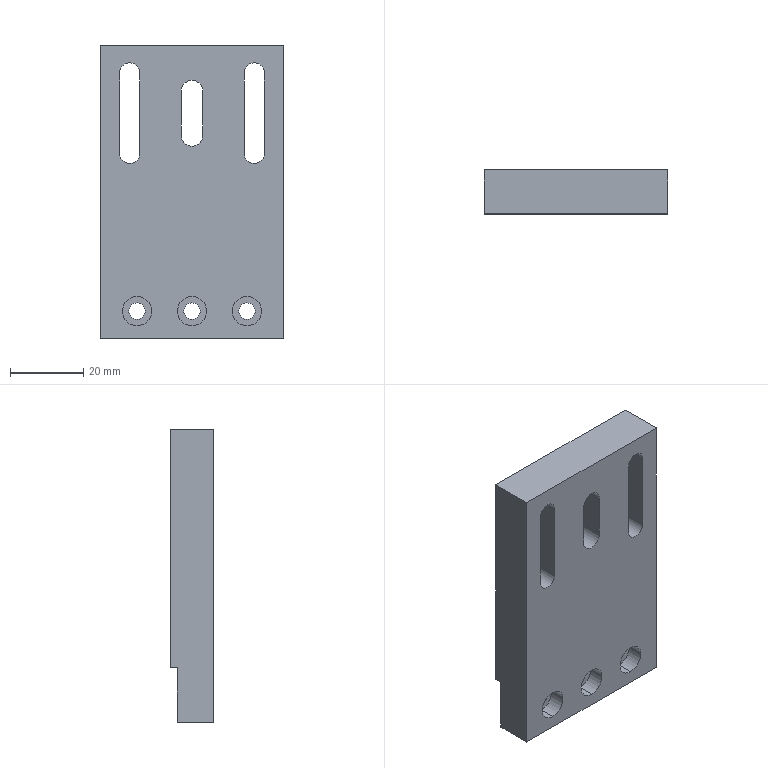Part | STEP file | 04-12 support plate | 1 solid | 50 faces | box 50 x 12 x 80 mm | volume 39354 mm3 | cylinder 27 | plane 23 | commonest cylinder face diameters 4.5 x6 5.5 x6 8 x6 10 x6 6 x3
STEP:
#1=CARTESIAN_POINT('',(17.,-6.,75.25));
#2=VERTEX_POINT('',#1);
#3=CARTESIAN_POINT('',(19.75,-6.,72.5));
#4=VERTEX_POINT('',#3);
#5=CARTESIAN_POINT('',(17.,-6.,72.5));
#6=DIRECTION('',(0.,1.,0.));
#7=DIRECTION('',(-1.,0.,0.));
#8=AXIS2_PLACEMENT_3D('',#5,#6,#7);
#9=CIRCLE('',#8,2.75);
#10=EDGE_CURVE('',#2,#4,#9,.T.);
#11=ORIENTED_EDGE('',*,*,#10,.F.);
#12=CARTESIAN_POINT('',(17.,1.,75.25));
#13=VERTEX_POINT('',#12);
#14=CARTESIAN_POINT('',(17.,-10.,75.25));
#15=DIRECTION('',(0.,1.,0.));
#16=VECTOR('',#15,1000.);
#17=LINE('',#14,#16);
#18=EDGE_CURVE('',#2,#13,#17,.T.);
#19=ORIENTED_EDGE('',*,*,#18,.T.);
#20=CARTESIAN_POINT('',(19.75,1.,72.5));
#21=VERTEX_POINT('',#20);
#22=CARTESIAN_POINT('',(17.,1.,72.5));
#23=DIRECTION('',(0.,-1.,0.));
#24=DIRECTION('',(0.,0.,-1.));
#25=AXIS2_PLACEMENT_3D('',#22,#23,#24);
#26=CIRCLE('',#25,2.75);
#27=EDGE_CURVE('',#21,#13,#26,.T.);
#28=ORIENTED_EDGE('',*,*,#27,.F.);
#29=CARTESIAN_POINT('',(19.75,-10.,72.5));
#30=DIRECTION('',(0.,1.,0.));
#31=VECTOR('',#30,1000.);
#32=LINE('',#29,#31);
#33=EDGE_CURVE('',#4,#21,#32,.T.);
#34=ORIENTED_EDGE('',*,*,#33,.F.);
#35=EDGE_LOOP('',(#11,#19,#28,#34));
#36=FACE_OUTER_BOUND('',#35,.T.);
#37=CARTESIAN_POINT('',(17.,-10.,72.5));
#38=DIRECTION('',(0.,1.,0.));
#39=DIRECTION('',(0.,0.,1.));
#40=AXIS2_PLACEMENT_3D('',#37,#38,#39);
#41=CYLINDRICAL_SURFACE('',#40,2.75);
#42=ADVANCED_FACE('',(#36),#41,.F.);
#43=CARTESIAN_POINT('',(-17.,-6.,75.25));
#44=VERTEX_POINT('',#43);
#45=CARTESIAN_POINT('',(-14.25,-6.,72.5));
#46=VERTEX_POINT('',#45);
#47=CARTESIAN_POINT('',(-17.,-6.,72.5));
#48=DIRECTION('',(0.,1.,0.));
#49=DIRECTION('',(-1.,0.,0.));
#50=AXIS2_PLACEMENT_3D('',#47,#48,#49);
#51=CIRCLE('',#50,2.75);
#52=EDGE_CURVE('',#44,#46,#51,.T.);
#53=ORIENTED_EDGE('',*,*,#52,.F.);
#54=CARTESIAN_POINT('',(-17.,1.,75.25));
#55=VERTEX_POINT('',#54);
#56=CARTESIAN_POINT('',(-17.,-10.,75.25));
#57=DIRECTION('',(0.,1.,0.));
#58=VECTOR('',#57,1000.);
#59=LINE('',#56,#58);
#60=EDGE_CURVE('',#44,#55,#59,.T.);
#61=ORIENTED_EDGE('',*,*,#60,.T.);
#62=CARTESIAN_POINT('',(-14.25,1.,72.5));
#63=VERTEX_POINT('',#62);
#64=CARTESIAN_POINT('',(-17.,1.,72.5));
#65=DIRECTION('',(0.,1.,0.));
#66=DIRECTION('',(0.,0.,1.));
#67=AXIS2_PLACEMENT_3D('',#64,#65,#66);
#68=CIRCLE('',#67,2.75);
#69=EDGE_CURVE('',#55,#63,#68,.T.);
#70=ORIENTED_EDGE('',*,*,#69,.T.);
#71=CARTESIAN_POINT('',(-14.25,-10.,72.5));
#72=DIRECTION('',(0.,1.,0.));
#73=VECTOR('',#72,1000.);
#74=LINE('',#71,#73);
#75=EDGE_CURVE('',#46,#63,#74,.T.);
#76=ORIENTED_EDGE('',*,*,#75,.F.);
#77=EDGE_LOOP('',(#53,#61,#70,#76));
#78=FACE_OUTER_BOUND('',#77,.T.);
#79=CARTESIAN_POINT('',(-17.,-10.,72.5));
#80=DIRECTION('',(0.,1.,0.));
#81=DIRECTION('',(0.,0.,1.));
#82=AXIS2_PLACEMENT_3D('',#79,#80,#81);
#83=CYLINDRICAL_SURFACE('',#82,2.75);
#84=ADVANCED_FACE('',(#78),#83,.F.);
#85=CARTESIAN_POINT('',(0.,-6.,70.5));
#86=VERTEX_POINT('',#85);
#87=CARTESIAN_POINT('',(3.,-6.,67.5));
#88=VERTEX_POINT('',#87);
#89=CARTESIAN_POINT('',(0.,-6.,67.5));
#90=DIRECTION('',(0.,1.,0.));
#91=DIRECTION('',(-1.,0.,0.));
#92=AXIS2_PLACEMENT_3D('',#89,#90,#91);
#93=CIRCLE('',#92,3.);
#94=EDGE_CURVE('',#86,#88,#93,.T.);
#95=ORIENTED_EDGE('',*,*,#94,.F.);
#96=CARTESIAN_POINT('',(0.,6.,70.5));
#97=VERTEX_POINT('',#96);
#98=CARTESIAN_POINT('',(0.,-10.,70.5));
#99=DIRECTION('',(0.,1.,0.));
#100=VECTOR('',#99,1000.);
#101=LINE('',#98,#100);
#102=EDGE_CURVE('',#86,#97,#101,.T.);
#103=ORIENTED_EDGE('',*,*,#102,.T.);
#104=CARTESIAN_POINT('',(3.,6.,67.5));
#105=VERTEX_POINT('',#104);
#106=CARTESIAN_POINT('',(0.,6.,67.5));
#107=DIRECTION('',(0.,-1.,0.));
#108=DIRECTION('',(0.,0.,-1.));
#109=AXIS2_PLACEMENT_3D('',#106,#107,#108);
#110=CIRCLE('',#109,3.);
#111=EDGE_CURVE('',#105,#97,#110,.T.);
#112=ORIENTED_EDGE('',*,*,#111,.F.);
#113=CARTESIAN_POINT('',(3.,-10.,67.5));
#114=DIRECTION('',(0.,1.,0.));
#115=VECTOR('',#114,1000.);
#116=LINE('',#113,#115);
#117=EDGE_CURVE('',#88,#105,#116,.T.);
#118=ORIENTED_EDGE('',*,*,#117,.F.);
#119=EDGE_LOOP('',(#95,#103,#112,#118));
#120=FACE_OUTER_BOUND('',#119,.T.);
#121=CARTESIAN_POINT('',(0.,-10.,67.5));
#122=DIRECTION('',(0.,1.,0.));
#123=DIRECTION('',(0.,0.,1.));
#124=AXIS2_PLACEMENT_3D('',#121,#122,#123);
#125=CYLINDRICAL_SURFACE('',#124,3.);
#126=ADVANCED_FACE('',(#120),#125,.F.);
#127=CARTESIAN_POINT('',(17.,1.,77.5));
#128=VERTEX_POINT('',#127);
#129=CARTESIAN_POINT('',(22.,1.,72.5));
#130=VERTEX_POINT('',#129);
#131=CARTESIAN_POINT('',(17.,1.,72.5));
#132=DIRECTION('',(0.,1.,0.));
#133=DIRECTION('',(0.,0.,-1.));
#134=AXIS2_PLACEMENT_3D('',#131,#132,#133);
#135=CIRCLE('',#134,5.);
#136=EDGE_CURVE('',#128,#130,#135,.T.);
#137=ORIENTED_EDGE('',*,*,#136,.F.);
#138=CARTESIAN_POINT('',(17.,6.,77.5));
#139=VERTEX_POINT('',#138);
#140=CARTESIAN_POINT('',(17.,1.,77.5));
#141=DIRECTION('',(0.,1.,0.));
#142=VECTOR('',#141,1000.);
#143=LINE('',#140,#142);
#144=EDGE_CURVE('',#128,#139,#143,.T.);
#145=ORIENTED_EDGE('',*,*,#144,.T.);
#146=CARTESIAN_POINT('',(22.,6.,72.5));
#147=VERTEX_POINT('',#146);
#148=CARTESIAN_POINT('',(17.,6.,72.5));
#149=DIRECTION('',(0.,1.,0.));
#150=DIRECTION('',(0.,0.,-1.));
#151=AXIS2_PLACEMENT_3D('',#148,#149,#150);
#152=CIRCLE('',#151,5.);
#153=EDGE_CURVE('',#139,#147,#152,.T.);
#154=ORIENTED_EDGE('',*,*,#153,.T.);
#155=CARTESIAN_POINT('',(22.,1.,72.5));
#156=DIRECTION('',(0.,1.,0.));
#157=VECTOR('',#156,1000.);
#158=LINE('',#155,#157);
#159=EDGE_CURVE('',#130,#147,#158,.T.);
#160=ORIENTED_EDGE('',*,*,#159,.F.);
#161=EDGE_LOOP('',(#137,#145,#154,#160));
#162=FACE_OUTER_BOUND('',#161,.T.);
#163=CARTESIAN_POINT('',(17.,1.,72.5));
#164=DIRECTION('',(0.,1.,0.));
#165=DIRECTION('',(0.,0.,1.));
#166=AXIS2_PLACEMENT_3D('',#163,#164,#165);
#167=CYLINDRICAL_SURFACE('',#166,5.);
#168=ADVANCED_FACE('',(#162),#167,.F.);
#169=CARTESIAN_POINT('',(-17.,1.,77.5));
#170=VERTEX_POINT('',#169);
#171=CARTESIAN_POINT('',(-12.,1.,72.5));
#172=VERTEX_POINT('',#171);
#173=CARTESIAN_POINT('',(-17.,1.,72.5));
#174=DIRECTION('',(0.,1.,0.));
#175=DIRECTION('',(0.,0.,1.));
#176=AXIS2_PLACEMENT_3D('',#173,#174,#175);
#177=CIRCLE('',#176,5.);
#178=EDGE_CURVE('',#170,#172,#177,.T.);
#179=ORIENTED_EDGE('',*,*,#178,.F.);
#180=CARTESIAN_POINT('',(-17.,6.,77.5));
#181=VERTEX_POINT('',#180);
#182=CARTESIAN_POINT('',(-17.,1.,77.5));
#183=DIRECTION('',(0.,1.,0.));
#184=VECTOR('',#183,1000.);
#185=LINE('',#182,#184);
#186=EDGE_CURVE('',#170,#181,#185,.T.);
#187=ORIENTED_EDGE('',*,*,#186,.T.);
#188=CARTESIAN_POINT('',(-12.,6.,72.5));
#189=VERTEX_POINT('',#188);
#190=CARTESIAN_POINT('',(-17.,6.,72.5));
#191=DIRECTION('',(0.,1.,0.));
#192=DIRECTION('',(0.,0.,1.));
#193=AXIS2_PLACEMENT_3D('',#190,#191,#192);
#194=CIRCLE('',#193,5.);
#195=EDGE_CURVE('',#181,#189,#194,.T.);
#196=ORIENTED_EDGE('',*,*,#195,.T.);
#197=CARTESIAN_POINT('',(-12.,1.,72.5));
#198=DIRECTION('',(0.,1.,0.));
#199=VECTOR('',#198,1000.);
#200=LINE('',#197,#199);
#201=EDGE_CURVE('',#172,#189,#200,.T.);
#202=ORIENTED_EDGE('',*,*,#201,.F.);
#203=EDGE_LOOP('',(#179,#187,#196,#202));
#204=FACE_OUTER_BOUND('',#203,.T.);
#205=CARTESIAN_POINT('',(-17.,1.,72.5));
#206=DIRECTION('',(0.,1.,0.));
#207=DIRECTION('',(0.,0.,1.));
#208=AXIS2_PLACEMENT_3D('',#205,#206,#207);
#209=CYLINDRICAL_SURFACE('',#208,5.);
#210=ADVANCED_FACE('',(#204),#209,.F.);
#211=CARTESIAN_POINT('',(15.,-1.6,11.5));
#212=VERTEX_POINT('',#211);
#213=CARTESIAN_POINT('',(15.,-1.6,3.5));
#214=VERTEX_POINT('',#213);
#215=CARTESIAN_POINT('',(15.,-1.6,7.5));
#216=DIRECTION('',(0.,-1.,0.));
#217=DIRECTION('',(0.,0.,-1.));
#218=AXIS2_PLACEMENT_3D('',#215,#216,#217);
#219=CIRCLE('',#218,4.);
#220=EDGE_CURVE('',#212,#214,#219,.T.);
#221=ORIENTED_EDGE('',*,*,#220,.F.);
#222=CARTESIAN_POINT('',(15.,-6.,11.5));
#223=VERTEX_POINT('',#222);
#224=CARTESIAN_POINT('',(15.,-6.,11.5));
#225=DIRECTION('',(0.,-1.,0.));
#226=VECTOR('',#225,1000.);
#227=LINE('',#224,#226);
#228=EDGE_CURVE('',#212,#223,#227,.T.);
#229=ORIENTED_EDGE('',*,*,#228,.T.);
#230=CARTESIAN_POINT('',(15.,-6.,3.5));
#231=VERTEX_POINT('',#230);
#232=CARTESIAN_POINT('',(15.,-6.,7.5));
#233=DIRECTION('',(0.,-1.,0.));
#234=DIRECTION('',(0.,0.,-1.));
#235=AXIS2_PLACEMENT_3D('',#232,#233,#234);
#236=CIRCLE('',#235,4.);
#237=EDGE_CURVE('',#223,#231,#236,.T.);
#238=ORIENTED_EDGE('',*,*,#237,.T.);
#239=CARTESIAN_POINT('',(15.,-6.,3.5));
#240=DIRECTION('',(0.,-1.,0.));
#241=VECTOR('',#240,1000.);
#242=LINE('',#239,#241);
#243=EDGE_CURVE('',#214,#231,#242,.T.);
#244=ORIENTED_EDGE('',*,*,#243,.F.);
#245=EDGE_LOOP('',(#221,#229,#238,#244));
#246=FACE_OUTER_BOUND('',#245,.T.);
#247=CARTESIAN_POINT('',(15.,-6.,7.5));
#248=DIRECTION('',(0.,-1.,0.));
#249=DIRECTION('',(0.,0.,-1.));
#250=AXIS2_PLACEMENT_3D('',#247,#248,#249);
#251=CYLINDRICAL_SURFACE('',#250,4.);
#252=ADVANCED_FACE('',(#246),#251,.F.);
#253=CARTESIAN_POINT('',(15.,4.,9.75));
#254=VERTEX_POINT('',#253);
#255=CARTESIAN_POINT('',(15.,4.,5.25));
#256=VERTEX_POINT('',#255);
#257=CARTESIAN_POINT('',(15.,4.,7.5));
#258=DIRECTION('',(0.,-1.,0.));
#259=DIRECTION('',(1.,0.,0.));
#260=AXIS2_PLACEMENT_3D('',#257,#258,#259);
#261=CIRCLE('',#260,2.25);
#262=EDGE_CURVE('',#254,#256,#261,.T.);
#263=ORIENTED_EDGE('',*,*,#262,.F.);
#264=CARTESIAN_POINT('',(15.,-1.6,9.75));
#265=VERTEX_POINT('',#264);
#266=CARTESIAN_POINT('',(15.,-6.,9.75));
#267=DIRECTION('',(0.,-1.,0.));
#268=VECTOR('',#267,1000.);
#269=LINE('',#266,#268);
#270=EDGE_CURVE('',#254,#265,#269,.T.);
#271=ORIENTED_EDGE('',*,*,#270,.T.);
#272=CARTESIAN_POINT('',(15.,-1.6,5.25));
#273=VERTEX_POINT('',#272);
#274=CARTESIAN_POINT('',(15.,-1.6,7.5));
#275=DIRECTION('',(0.,-1.,0.));
#276=DIRECTION('',(0.,0.,-1.));
#277=AXIS2_PLACEMENT_3D('',#274,#275,#276);
#278=CIRCLE('',#277,2.25);
#279=EDGE_CURVE('',#265,#273,#278,.T.);
#280=ORIENTED_EDGE('',*,*,#279,.T.);
#281=CARTESIAN_POINT('',(15.,-6.,5.25));
#282=DIRECTION('',(0.,-1.,0.));
#283=VECTOR('',#282,1000.);
#284=LINE('',#281,#283);
#285=EDGE_CURVE('',#256,#273,#284,.T.);
#286=ORIENTED_EDGE('',*,*,#285,.F.);
#287=EDGE_LOOP('',(#263,#271,#280,#286));
#288=FACE_OUTER_BOUND('',#287,.T.);
#289=CARTESIAN_POINT('',(15.,-6.,7.5));
#290=DIRECTION('',(0.,-1.,0.));
#291=DIRECTION('',(0.,0.,-1.));
#292=AXIS2_PLACEMENT_3D('',#289,#290,#291);
#293=CYLINDRICAL_SURFACE('',#292,2.25);
#294=ADVANCED_FACE('',(#288),#293,.F.);
#295=CARTESIAN_POINT('',(0.,-1.6,11.5));
#296=VERTEX_POINT('',#295);
#297=CARTESIAN_POINT('',(0.,-1.6,3.5));
#298=VERTEX_POINT('',#297);
#299=CARTESIAN_POINT('',(0.,-1.6,7.5));
#300=DIRECTION('',(0.,-1.,0.));
#301=DIRECTION('',(0.,0.,-1.));
#302=AXIS2_PLACEMENT_3D('',#299,#300,#301);
#303=CIRCLE('',#302,4.);
#304=EDGE_CURVE('',#296,#298,#303,.T.);
#305=ORIENTED_EDGE('',*,*,#304,.F.);
#306=CARTESIAN_POINT('',(0.,-6.,11.5));
#307=VERTEX_POINT('',#306);
#308=CARTESIAN_POINT('',(0.,-6.,11.5));
#309=DIRECTION('',(0.,-1.,0.));
#310=VECTOR('',#309,1000.);
#311=LINE('',#308,#310);
#312=EDGE_CURVE('',#296,#307,#311,.T.);
#313=ORIENTED_EDGE('',*,*,#312,.T.);
#314=CARTESIAN_POINT('',(0.,-6.,3.5));
#315=VERTEX_POINT('',#314);
#316=CARTESIAN_POINT('',(0.,-6.,7.5));
#317=DIRECTION('',(0.,-1.,0.));
#318=DIRECTION('',(0.,0.,-1.));
#319=AXIS2_PLACEMENT_3D('',#316,#317,#318);
#320=CIRCLE('',#319,4.);
#321=EDGE_CURVE('',#307,#315,#320,.T.);
#322=ORIENTED_EDGE('',*,*,#321,.T.);
#323=CARTESIAN_POINT('',(0.,-6.,3.5));
#324=DIRECTION('',(0.,-1.,0.));
#325=VECTOR('',#324,1000.);
#326=LINE('',#323,#325);
#327=EDGE_CURVE('',#298,#315,#326,.T.);
#328=ORIENTED_EDGE('',*,*,#327,.F.);
#329=EDGE_LOOP('',(#305,#313,#322,#328));
#330=FACE_OUTER_BOUND('',#329,.T.);
#331=CARTESIAN_POINT('',(0.,-6.,7.5));
#332=DIRECTION('',(0.,-1.,0.));
#333=DIRECTION('',(0.,0.,-1.));
#334=AXIS2_PLACEMENT_3D('',#331,#332,#333);
#335=CYLINDRICAL_SURFACE('',#334,4.);
#336=ADVANCED_FACE('',(#330),#335,.F.);
#337=CARTESIAN_POINT('',(0.,4.,9.75));
#338=VERTEX_POINT('',#337);
#339=CARTESIAN_POINT('',(0.,4.,5.25));
#340=VERTEX_POINT('',#339);
#341=CARTESIAN_POINT('',(0.,4.,7.5));
#342=DIRECTION('',(0.,-1.,0.));
#343=DIRECTION('',(1.,0.,0.));
#344=AXIS2_PLACEMENT_3D('',#341,#342,#343);
#345=CIRCLE('',#344,2.25);
#346=EDGE_CURVE('',#338,#340,#345,.T.);
#347=ORIENTED_EDGE('',*,*,#346,.F.);
#348=CARTESIAN_POINT('',(0.,-1.6,9.75));
#349=VERTEX_POINT('',#348);
#350=CARTESIAN_POINT('',(0.,-6.,9.75));
#351=DIRECTION('',(0.,-1.,0.));
#352=VECTOR('',#351,1000.);
#353=LINE('',#350,#352);
#354=EDGE_CURVE('',#338,#349,#353,.T.);
#355=ORIENTED_EDGE('',*,*,#354,.T.);
#356=CARTESIAN_POINT('',(0.,-1.6,5.25));
#357=VERTEX_POINT('',#356);
#358=CARTESIAN_POINT('',(0.,-1.6,7.5));
#359=DIRECTION('',(0.,-1.,0.));
#360=DIRECTION('',(0.,0.,-1.));
#361=AXIS2_PLACEMENT_3D('',#358,#359,#360);
#362=CIRCLE('',#361,2.25);
#363=EDGE_CURVE('',#349,#357,#362,.T.);
#364=ORIENTED_EDGE('',*,*,#363,.T.);
#365=CARTESIAN_POINT('',(0.,-6.,5.25));
#366=DIRECTION('',(0.,-1.,0.));
#367=VECTOR('',#366,1000.);
#368=LINE('',#365,#367);
#369=EDGE_CURVE('',#340,#357,#368,.T.);
#370=ORIENTED_EDGE('',*,*,#369,.F.);
#371=EDGE_LOOP('',(#347,#355,#364,#370));
#372=FACE_OUTER_BOUND('',#371,.T.);
#373=CARTESIAN_POINT('',(0.,-6.,7.5));
#374=DIRECTION('',(0.,-1.,0.));
#375=DIRECTION('',(0.,0.,-1.));
#376=AXIS2_PLACEMENT_3D('',#373,#374,#375);
#377=CYLINDRICAL_SURFACE('',#376,2.25);
#378=ADVANCED_FACE('',(#372),#377,.F.);
#379=CARTESIAN_POINT('',(-15.,-1.6,11.5));
#380=VERTEX_POINT('',#379);
#381=CARTESIAN_POINT('',(-15.,-1.6,3.5));
#382=VERTEX_POINT('',#381);
#383=CARTESIAN_POINT('',(-15.,-1.6,7.5));
#384=DIRECTION('',(0.,-1.,0.));
#385=DIRECTION('',(0.,0.,-1.));
#386=AXIS2_PLACEMENT_3D('',#383,#384,#385);
#387=CIRCLE('',#386,4.);
#388=EDGE_CURVE('',#380,#382,#387,.T.);
#389=ORIENTED_EDGE('',*,*,#388,.F.);
#390=CARTESIAN_POINT('',(-15.,-6.,11.5));
#391=VERTEX_POINT('',#390);
#392=CARTESIAN_POINT('',(-15.,-6.,11.5));
#393=DIRECTION('',(0.,-1.,0.));
#394=VECTOR('',#393,1000.);
#395=LINE('',#392,#394);
#396=EDGE_CURVE('',#380,#391,#395,.T.);
#397=ORIENTED_EDGE('',*,*,#396,.T.);
#398=CARTESIAN_POINT('',(-15.,-6.,3.5));
#399=VERTEX_POINT('',#398);
#400=CARTESIAN_POINT('',(-15.,-6.,7.5));
#401=DIRECTION('',(0.,-1.,0.));
#402=DIRECTION('',(0.,0.,-1.));
#403=AXIS2_PLACEMENT_3D('',#400,#401,#402);
#404=CIRCLE('',#403,4.);
#405=EDGE_CURVE('',#391,#399,#404,.T.);
#406=ORIENTED_EDGE('',*,*,#405,.T.);
#407=CARTESIAN_POINT('',(-15.,-6.,3.5));
#408=DIRECTION('',(0.,-1.,0.));
#409=VECTOR('',#408,1000.);
#410=LINE('',#407,#409);
#411=EDGE_CURVE('',#382,#399,#410,.T.);
#412=ORIENTED_EDGE('',*,*,#411,.F.);
#413=EDGE_LOOP('',(#389,#397,#406,#412));
#414=FACE_OUTER_BOUND('',#413,.T.);
#415=CARTESIAN_POINT('',(-15.,-6.,7.5));
#416=DIRECTION('',(0.,-1.,0.));
#417=DIRECTION('',(0.,0.,-1.));
#418=AXIS2_PLACEMENT_3D('',#415,#416,#417);
#419=CYLINDRICAL_SURFACE('',#418,4.);
#420=ADVANCED_FACE('',(#414),#419,.F.);
#421=CARTESIAN_POINT('',(-15.,4.,9.75));
#422=VERTEX_POINT('',#421);
#423=CARTESIAN_POINT('',(-15.,4.,5.25));
#424=VERTEX_POINT('',#423);
#425=CARTESIAN_POINT('',(-15.,4.,7.5));
#426=DIRECTION('',(0.,-1.,0.));
#427=DIRECTION('',(1.,0.,0.));
#428=AXIS2_PLACEMENT_3D('',#425,#426,#427);
#429=CIRCLE('',#428,2.25);
#430=EDGE_CURVE('',#422,#424,#429,.T.);
#431=ORIENTED_EDGE('',*,*,#430,.F.);
#432=CARTESIAN_POINT('',(-15.,-1.6,9.75));
#433=VERTEX_POINT('',#432);
#434=CARTESIAN_POINT('',(-15.,-6.,9.75));
#435=DIRECTION('',(0.,-1.,0.));
#436=VECTOR('',#435,1000.);
#437=LINE('',#434,#436);
#438=EDGE_CURVE('',#422,#433,#437,.T.);
#439=ORIENTED_EDGE('',*,*,#438,.T.);
#440=CARTESIAN_POINT('',(-15.,-1.6,5.25));
#441=VERTEX_POINT('',#440);
#442=CARTESIAN_POINT('',(-15.,-1.6,7.5));
#443=DIRECTION('',(0.,-1.,0.));
#444=DIRECTION('',(0.,0.,-1.));
#445=AXIS2_PLACEMENT_3D('',#442,#443,#444);
#446=CIRCLE('',#445,2.25);
#447=EDGE_CURVE('',#433,#441,#446,.T.);
#448=ORIENTED_EDGE('',*,*,#447,.T.);
#449=CARTESIAN_POINT('',(-15.,-6.,5.25));
#450=DIRECTION('',(0.,-1.,0.));
#451=VECTOR('',#450,1000.);
#452=LINE('',#449,#451);
#453=EDGE_CURVE('',#424,#441,#452,.T.);
#454=ORIENTED_EDGE('',*,*,#453,.F.);
#455=EDGE_LOOP('',(#431,#439,#448,#454));
#456=FACE_OUTER_BOUND('',#455,.T.);
#457=CARTESIAN_POINT('',(-15.,-6.,7.5));
#458=DIRECTION('',(0.,-1.,0.));
#459=DIRECTION('',(0.,0.,-1.));
#460=AXIS2_PLACEMENT_3D('',#457,#458,#459);
#461=CYLINDRICAL_SURFACE('',#460,2.25);
#462=ADVANCED_FACE('',(#456),#461,.F.);
#463=CARTESIAN_POINT('',(25.,-6.,0.));
#464=VERTEX_POINT('',#463);
#465=CARTESIAN_POINT('',(25.,4.,0.));
#466=VERTEX_POINT('',#465);
#467=CARTESIAN_POINT('',(25.,6.,0.));
#468=DIRECTION('',(0.,1.,0.));
#469=VECTOR('',#468,1000.);
#470=LINE('',#467,#469);
#471=EDGE_CURVE('',#464,#466,#470,.T.);
#472=ORIENTED_EDGE('',*,*,#471,.T.);
#473=CARTESIAN_POINT('',(25.,4.,15.));
#474=VERTEX_POINT('',#473);
#475=CARTESIAN_POINT('',(25.,4.,0.));
#476=DIRECTION('',(0.,0.,-1.));
#477=VECTOR('',#476,1000.);
#478=LINE('',#475,#477);
#479=EDGE_CURVE('',#474,#466,#478,.T.);
#480=ORIENTED_EDGE('',*,*,#479,.F.);
#481=CARTESIAN_POINT('',(25.,6.,15.));
#482=VERTEX_POINT('',#481);
#483=CARTESIAN_POINT('',(25.,6.,15.));
#484=DIRECTION('',(0.,-1.,0.));
#485=VECTOR('',#484,1000.);
#486=LINE('',#483,#485);
#487=EDGE_CURVE('',#482,#474,#486,.T.);
#488=ORIENTED_EDGE('',*,*,#487,.F.);
#489=CARTESIAN_POINT('',(25.,6.,80.));
#490=VERTEX_POINT('',#489);
#491=CARTESIAN_POINT('',(25.,6.,80.));
#492=DIRECTION('',(0.,0.,-1.));
#493=VECTOR('',#492,1000.);
#494=LINE('',#491,#493);
#495=EDGE_CURVE('',#490,#482,#494,.T.);
#496=ORIENTED_EDGE('',*,*,#495,.F.);
#497=CARTESIAN_POINT('',(25.,-6.,80.));
#498=VERTEX_POINT('',#497);
#499=CARTESIAN_POINT('',(25.,6.,80.));
#500=DIRECTION('',(0.,1.,0.));
#501=VECTOR('',#500,1000.);
#502=LINE('',#499,#501);
#503=EDGE_CURVE('',#498,#490,#502,.T.);
#504=ORIENTED_EDGE('',*,*,#503,.F.);
#505=CARTESIAN_POINT('',(25.,-6.,80.));
#506=DIRECTION('',(0.,0.,-1.));
#507=VECTOR('',#506,1000.);
#508=LINE('',#505,#507);
#509=EDGE_CURVE('',#498,#464,#508,.T.);
#510=ORIENTED_EDGE('',*,*,#509,.T.);
#511=EDGE_LOOP('',(#472,#480,#488,#496,#504,#510));
#512=FACE_OUTER_BOUND('',#511,.T.);
#513=CARTESIAN_POINT('',(25.,6.,80.));
#514=DIRECTION('',(-1.,0.,0.));
#515=DIRECTION('',(0.,-1.,0.));
#516=AXIS2_PLACEMENT_3D('',#513,#514,#515);
#517=PLANE('',#516);
#518=ADVANCED_FACE('',(#512),#517,.F.);
#519=CARTESIAN_POINT('',(-3.,6.,67.5));
#520=VERTEX_POINT('',#519);
#521=CARTESIAN_POINT('',(-3.,6.,55.5));
#522=VERTEX_POINT('',#521);
#523=CARTESIAN_POINT('',(-3.,6.,80.));
#524=DIRECTION('',(0.,0.,-1.));
#525=VECTOR('',#524,1000.);
#526=LINE('',#523,#525);
#527=EDGE_CURVE('',#520,#522,#526,.T.);
#528=ORIENTED_EDGE('',*,*,#527,.T.);
#529=CARTESIAN_POINT('',(3.,6.,55.5));
#530=VERTEX_POINT('',#529);
#531=CARTESIAN_POINT('',(0.,6.,55.5));
#532=DIRECTION('',(0.,-1.,0.));
#533=DIRECTION('',(0.,0.,-1.));
#534=AXIS2_PLACEMENT_3D('',#531,#532,#533);
#535=CIRCLE('',#534,3.);
#536=EDGE_CURVE('',#522,#530,#535,.T.);
#537=ORIENTED_EDGE('',*,*,#536,.T.);
#538=CARTESIAN_POINT('',(3.,6.,80.));
#539=DIRECTION('',(0.,0.,1.));
#540=VECTOR('',#539,1000.);
#541=LINE('',#538,#540);
#542=EDGE_CURVE('',#530,#105,#541,.T.);
#543=ORIENTED_EDGE('',*,*,#542,.T.);
#544=ORIENTED_EDGE('',*,*,#111,.T.);
#545=CARTESIAN_POINT('',(0.,6.,67.5));
#546=DIRECTION('',(0.,-1.,0.));
#547=DIRECTION('',(0.,0.,-1.));
#548=AXIS2_PLACEMENT_3D('',#545,#546,#547);
#549=CIRCLE('',#548,3.);
#550=EDGE_CURVE('',#97,#520,#549,.T.);
#551=ORIENTED_EDGE('',*,*,#550,.T.);
#552=EDGE_LOOP('',(#528,#537,#543,#544,#551));
#553=FACE_BOUND('',#552,.T.);
#554=CARTESIAN_POINT('',(12.,6.,50.5));
#555=VERTEX_POINT('',#554);
#556=CARTESIAN_POINT('',(12.,6.,72.5));
#557=VERTEX_POINT('',#556);
#558=CARTESIAN_POINT('',(12.,6.,50.5));
#559=DIRECTION('',(0.,0.,1.));
#560=VECTOR('',#559,1000.);
#561=LINE('',#558,#560);
#562=EDGE_CURVE('',#555,#557,#561,.T.);
#563=ORIENTED_EDGE('',*,*,#562,.F.);
#564=CARTESIAN_POINT('',(22.,6.,50.5));
#565=VERTEX_POINT('',#564);
#566=CARTESIAN_POINT('',(17.,6.,50.5));
#567=DIRECTION('',(0.,1.,0.));
#568=DIRECTION('',(0.,0.,-1.));
#569=AXIS2_PLACEMENT_3D('',#566,#567,#568);
#570=CIRCLE('',#569,5.);
#571=EDGE_CURVE('',#565,#555,#570,.T.);
#572=ORIENTED_EDGE('',*,*,#571,.F.);
#573=CARTESIAN_POINT('',(22.,6.,50.5));
#574=DIRECTION('',(0.,0.,-1.));
#575=VECTOR('',#574,1000.);
#576=LINE('',#573,#575);
#577=EDGE_CURVE('',#147,#565,#576,.T.);
#578=ORIENTED_EDGE('',*,*,#577,.F.);
#579=ORIENTED_EDGE('',*,*,#153,.F.);
#580=CARTESIAN_POINT('',(17.,6.,72.5));
#581=DIRECTION('',(0.,1.,0.));
#582=DIRECTION('',(0.,0.,-1.));
#583=AXIS2_PLACEMENT_3D('',#580,#581,#582);
#584=CIRCLE('',#583,5.);
#585=EDGE_CURVE('',#557,#139,#584,.T.);
#586=ORIENTED_EDGE('',*,*,#585,.F.);
#587=EDGE_LOOP('',(#563,#572,#578,#579,#586));
#588=FACE_BOUND('',#587,.T.);
#589=CARTESIAN_POINT('',(-22.,6.,50.5));
#590=VERTEX_POINT('',#589);
#591=CARTESIAN_POINT('',(-22.,6.,72.5));
#592=VERTEX_POINT('',#591);
#593=CARTESIAN_POINT('',(-22.,6.,50.5));
#594=DIRECTION('',(0.,0.,1.));
#595=VECTOR('',#594,1000.);
#596=LINE('',#593,#595);
#597=EDGE_CURVE('',#590,#592,#596,.T.);
#598=ORIENTED_EDGE('',*,*,#597,.F.);
#599=CARTESIAN_POINT('',(-12.,6.,50.5));
#600=VERTEX_POINT('',#599);
#601=CARTESIAN_POINT('',(-17.,6.,50.5));
#602=DIRECTION('',(0.,1.,0.));
#603=DIRECTION('',(0.,0.,1.));
#604=AXIS2_PLACEMENT_3D('',#601,#602,#603);
#605=CIRCLE('',#604,5.);
#606=EDGE_CURVE('',#600,#590,#605,.T.);
#607=ORIENTED_EDGE('',*,*,#606,.F.);
#608=CARTESIAN_POINT('',(-12.,6.,50.5));
#609=DIRECTION('',(0.,0.,-1.));
#610=VECTOR('',#609,1000.);
#611=LINE('',#608,#610);
#612=EDGE_CURVE('',#189,#600,#611,.T.);
#613=ORIENTED_EDGE('',*,*,#612,.F.);
#614=ORIENTED_EDGE('',*,*,#195,.F.);
#615=CARTESIAN_POINT('',(-17.,6.,72.5));
#616=DIRECTION('',(0.,1.,0.));
#617=DIRECTION('',(0.,0.,1.));
#618=AXIS2_PLACEMENT_3D('',#615,#616,#617);
#619=CIRCLE('',#618,5.);
#620=EDGE_CURVE('',#592,#181,#619,.T.);
#621=ORIENTED_EDGE('',*,*,#620,.F.);
#622=EDGE_LOOP('',(#598,#607,#613,#614,#621));
#623=FACE_BOUND('',#622,.T.);
#624=ORIENTED_EDGE('',*,*,#495,.T.);
#625=CARTESIAN_POINT('',(-25.,6.,15.));
#626=VERTEX_POINT('',#625);
#627=CARTESIAN_POINT('',(-35.,6.,15.));
#628=DIRECTION('',(1.,0.,0.));
#629=VECTOR('',#628,1000.);
#630=LINE('',#627,#629);
#631=EDGE_CURVE('',#626,#482,#630,.T.);
#632=ORIENTED_EDGE('',*,*,#631,.F.);
#633=CARTESIAN_POINT('',(-25.,6.,80.));
#634=VERTEX_POINT('',#633);
#635=CARTESIAN_POINT('',(-25.,6.,80.));
#636=DIRECTION('',(0.,0.,-1.));
#637=VECTOR('',#636,1000.);
#638=LINE('',#635,#637);
#639=EDGE_CURVE('',#634,#626,#638,.T.);
#640=ORIENTED_EDGE('',*,*,#639,.F.);
#641=CARTESIAN_POINT('',(-25.,6.,80.));
#642=DIRECTION('',(-1.,0.,0.));
#643=VECTOR('',#642,1000.);
#644=LINE('',#641,#643);
#645=EDGE_CURVE('',#490,#634,#644,.T.);
#646=ORIENTED_EDGE('',*,*,#645,.F.);
#647=EDGE_LOOP('',(#624,#632,#640,#646));
#648=FACE_OUTER_BOUND('',#647,.T.);
#649=CARTESIAN_POINT('',(-25.,6.,80.));
#650=DIRECTION('',(0.,-1.,0.));
#651=DIRECTION('',(0.,0.,-1.));
#652=AXIS2_PLACEMENT_3D('',#649,#650,#651);
#653=PLANE('',#652);
#654=ADVANCED_FACE('',(#553,#588,#623,#648),#653,.F.);
#655=CARTESIAN_POINT('',(-25.,4.,15.));
#656=VERTEX_POINT('',#655);
#657=CARTESIAN_POINT('',(-25.,6.,15.));
#658=DIRECTION('',(0.,-1.,0.));
#659=VECTOR('',#658,1000.);
#660=LINE('',#657,#659);
#661=EDGE_CURVE('',#626,#656,#660,.T.);
#662=ORIENTED_EDGE('',*,*,#661,.T.);
#663=CARTESIAN_POINT('',(-25.,4.,0.));
#664=VERTEX_POINT('',#663);
#665=CARTESIAN_POINT('',(-25.,4.,80.));
#666=DIRECTION('',(0.,0.,-1.));
#667=VECTOR('',#666,1000.);
#668=LINE('',#665,#667);
#669=EDGE_CURVE('',#656,#664,#668,.T.);
#670=ORIENTED_EDGE('',*,*,#669,.T.);
#671=CARTESIAN_POINT('',(-25.,-6.,0.));
#672=VERTEX_POINT('',#671);
#673=CARTESIAN_POINT('',(-25.,6.,0.));
#674=DIRECTION('',(0.,-1.,0.));
#675=VECTOR('',#674,1000.);
#676=LINE('',#673,#675);
#677=EDGE_CURVE('',#664,#672,#676,.T.);
#678=ORIENTED_EDGE('',*,*,#677,.T.);
#679=CARTESIAN_POINT('',(-25.,-6.,80.));
#680=VERTEX_POINT('',#679);
#681=CARTESIAN_POINT('',(-25.,-6.,80.));
#682=DIRECTION('',(0.,0.,-1.));
#683=VECTOR('',#682,1000.);
#684=LINE('',#681,#683);
#685=EDGE_CURVE('',#680,#672,#684,.T.);
#686=ORIENTED_EDGE('',*,*,#685,.F.);
#687=CARTESIAN_POINT('',(-25.,6.,80.));
#688=DIRECTION('',(0.,-1.,0.));
#689=VECTOR('',#688,1000.);
#690=LINE('',#687,#689);
#691=EDGE_CURVE('',#634,#680,#690,.T.);
#692=ORIENTED_EDGE('',*,*,#691,.F.);
#693=ORIENTED_EDGE('',*,*,#639,.T.);
#694=EDGE_LOOP('',(#662,#670,#678,#686,#692,#693));
#695=FACE_OUTER_BOUND('',#694,.T.);
#696=CARTESIAN_POINT('',(-25.,6.,80.));
#697=DIRECTION('',(1.,0.,0.));
#698=DIRECTION('',(0.,0.,-1.));
#699=AXIS2_PLACEMENT_3D('',#696,#697,#698);
#700=PLANE('',#699);
#701=ADVANCED_FACE('',(#695),#700,.F.);
#702=CARTESIAN_POINT('',(19.75,-6.,50.5));
#703=VERTEX_POINT('',#702);
#704=CARTESIAN_POINT('',(19.75,-6.,80.));
#705=DIRECTION('',(0.,0.,-1.));
#706=VECTOR('',#705,1000.);
#707=LINE('',#704,#706);
#708=EDGE_CURVE('',#4,#703,#707,.T.);
#709=ORIENTED_EDGE('',*,*,#708,.T.);
#710=CARTESIAN_POINT('',(14.25,-6.,50.5));
#711=VERTEX_POINT('',#710);
#712=CARTESIAN_POINT('',(17.,-6.,50.5));
#713=DIRECTION('',(0.,1.,0.));
#714=DIRECTION('',(-1.,0.,0.));
#715=AXIS2_PLACEMENT_3D('',#712,#713,#714);
#716=CIRCLE('',#715,2.75);
#717=EDGE_CURVE('',#703,#711,#716,.T.);
#718=ORIENTED_EDGE('',*,*,#717,.T.);
#719=CARTESIAN_POINT('',(14.25,-6.,72.5));
#720=VERTEX_POINT('',#719);
#721=CARTESIAN_POINT('',(14.25,-6.,80.));
#722=DIRECTION('',(0.,0.,1.));
#723=VECTOR('',#722,1000.);
#724=LINE('',#721,#723);
#725=EDGE_CURVE('',#711,#720,#724,.T.);
#726=ORIENTED_EDGE('',*,*,#725,.T.);
#727=CARTESIAN_POINT('',(17.,-6.,72.5));
#728=DIRECTION('',(0.,1.,0.));
#729=DIRECTION('',(-1.,0.,0.));
#730=AXIS2_PLACEMENT_3D('',#727,#728,#729);
#731=CIRCLE('',#730,2.75);
#732=EDGE_CURVE('',#720,#2,#731,.T.);
#733=ORIENTED_EDGE('',*,*,#732,.T.);
#734=ORIENTED_EDGE('',*,*,#10,.T.);
#735=EDGE_LOOP('',(#709,#718,#726,#733,#734));
#736=FACE_BOUND('',#735,.T.);
#737=CARTESIAN_POINT('',(-14.25,-6.,50.5));
#738=VERTEX_POINT('',#737);
#739=CARTESIAN_POINT('',(-14.25,-6.,80.));
#740=DIRECTION('',(0.,0.,-1.));
#741=VECTOR('',#740,1000.);
#742=LINE('',#739,#741);
#743=EDGE_CURVE('',#46,#738,#742,.T.);
#744=ORIENTED_EDGE('',*,*,#743,.T.);
#745=CARTESIAN_POINT('',(-19.75,-6.,50.5));
#746=VERTEX_POINT('',#745);
#747=CARTESIAN_POINT('',(-17.,-6.,50.5));
#748=DIRECTION('',(0.,1.,0.));
#749=DIRECTION('',(-1.,0.,0.));
#750=AXIS2_PLACEMENT_3D('',#747,#748,#749);
#751=CIRCLE('',#750,2.75);
#752=EDGE_CURVE('',#738,#746,#751,.T.);
#753=ORIENTED_EDGE('',*,*,#752,.T.);
#754=CARTESIAN_POINT('',(-19.75,-6.,72.5));
#755=VERTEX_POINT('',#754);
#756=CARTESIAN_POINT('',(-19.75,-6.,80.));
#757=DIRECTION('',(0.,0.,1.));
#758=VECTOR('',#757,1000.);
#759=LINE('',#756,#758);
#760=EDGE_CURVE('',#746,#755,#759,.T.);
#761=ORIENTED_EDGE('',*,*,#760,.T.);
#762=CARTESIAN_POINT('',(-17.,-6.,72.5));
#763=DIRECTION('',(0.,1.,0.));
#764=DIRECTION('',(-1.,0.,0.));
#765=AXIS2_PLACEMENT_3D('',#762,#763,#764);
#766=CIRCLE('',#765,2.75);
#767=EDGE_CURVE('',#755,#44,#766,.T.);
#768=ORIENTED_EDGE('',*,*,#767,.T.);
#769=ORIENTED_EDGE('',*,*,#52,.T.);
#770=EDGE_LOOP('',(#744,#753,#761,#768,#769));
#771=FACE_BOUND('',#770,.T.);
#772=CARTESIAN_POINT('',(3.,-6.,55.5));
#773=VERTEX_POINT('',#772);
#774=CARTESIAN_POINT('',(3.,-6.,80.));
#775=DIRECTION('',(0.,0.,-1.));
#776=VECTOR('',#775,1000.);
#777=LINE('',#774,#776);
#778=EDGE_CURVE('',#88,#773,#777,.T.);
#779=ORIENTED_EDGE('',*,*,#778,.T.);
#780=CARTESIAN_POINT('',(-3.,-6.,55.5));
#781=VERTEX_POINT('',#780);
#782=CARTESIAN_POINT('',(0.,-6.,55.5));
#783=DIRECTION('',(0.,1.,0.));
#784=DIRECTION('',(-1.,0.,0.));
#785=AXIS2_PLACEMENT_3D('',#782,#783,#784);
#786=CIRCLE('',#785,3.);
#787=EDGE_CURVE('',#773,#781,#786,.T.);
#788=ORIENTED_EDGE('',*,*,#787,.T.);
#789=CARTESIAN_POINT('',(-3.,-6.,67.5));
#790=VERTEX_POINT('',#789);
#791=CARTESIAN_POINT('',(-3.,-6.,80.));
#792=DIRECTION('',(0.,0.,1.));
#793=VECTOR('',#792,1000.);
#794=LINE('',#791,#793);
#795=EDGE_CURVE('',#781,#790,#794,.T.);
#796=ORIENTED_EDGE('',*,*,#795,.T.);
#797=CARTESIAN_POINT('',(0.,-6.,67.5));
#798=DIRECTION('',(0.,1.,0.));
#799=DIRECTION('',(-1.,0.,0.));
#800=AXIS2_PLACEMENT_3D('',#797,#798,#799);
#801=CIRCLE('',#800,3.);
#802=EDGE_CURVE('',#790,#86,#801,.T.);
#803=ORIENTED_EDGE('',*,*,#802,.T.);
#804=ORIENTED_EDGE('',*,*,#94,.T.);
#805=EDGE_LOOP('',(#779,#788,#796,#803,#804));
#806=FACE_BOUND('',#805,.T.);
#807=CARTESIAN_POINT('',(15.,-6.,7.5));
#808=DIRECTION('',(0.,-1.,0.));
#809=DIRECTION('',(0.,0.,-1.));
#810=AXIS2_PLACEMENT_3D('',#807,#808,#809);
#811=CIRCLE('',#810,4.);
#812=EDGE_CURVE('',#231,#223,#811,.T.);
#813=ORIENTED_EDGE('',*,*,#812,.F.);
#814=ORIENTED_EDGE('',*,*,#237,.F.);
#815=EDGE_LOOP('',(#813,#814));
#816=FACE_BOUND('',#815,.T.);
#817=CARTESIAN_POINT('',(0.,-6.,7.5));
#818=DIRECTION('',(0.,-1.,0.));
#819=DIRECTION('',(0.,0.,-1.));
#820=AXIS2_PLACEMENT_3D('',#817,#818,#819);
#821=CIRCLE('',#820,4.);
#822=EDGE_CURVE('',#315,#307,#821,.T.);
#823=ORIENTED_EDGE('',*,*,#822,.F.);
#824=ORIENTED_EDGE('',*,*,#321,.F.);
#825=EDGE_LOOP('',(#823,#824));
#826=FACE_BOUND('',#825,.T.);
#827=CARTESIAN_POINT('',(-15.,-6.,7.5));
#828=DIRECTION('',(0.,-1.,0.));
#829=DIRECTION('',(0.,0.,-1.));
#830=AXIS2_PLACEMENT_3D('',#827,#828,#829);
#831=CIRCLE('',#830,4.);
#832=EDGE_CURVE('',#399,#391,#831,.T.);
#833=ORIENTED_EDGE('',*,*,#832,.F.);
#834=ORIENTED_EDGE('',*,*,#405,.F.);
#835=EDGE_LOOP('',(#833,#834));
#836=FACE_BOUND('',#835,.T.);
#837=CARTESIAN_POINT('',(-25.,-6.,0.));
#838=DIRECTION('',(1.,0.,0.));
#839=VECTOR('',#838,1000.);
#840=LINE('',#837,#839);
#841=EDGE_CURVE('',#672,#464,#840,.T.);
#842=ORIENTED_EDGE('',*,*,#841,.T.);
#843=ORIENTED_EDGE('',*,*,#509,.F.);
#844=CARTESIAN_POINT('',(-25.,-6.,80.));
#845=DIRECTION('',(1.,0.,0.));
#846=VECTOR('',#845,1000.);
#847=LINE('',#844,#846);
#848=EDGE_CURVE('',#680,#498,#847,.T.);
#849=ORIENTED_EDGE('',*,*,#848,.F.);
#850=ORIENTED_EDGE('',*,*,#685,.T.);
#851=EDGE_LOOP('',(#842,#843,#849,#850));
#852=FACE_OUTER_BOUND('',#851,.T.);
#853=CARTESIAN_POINT('',(-25.,-6.,80.));
#854=DIRECTION('',(0.,1.,0.));
#855=DIRECTION('',(-1.,0.,0.));
#856=AXIS2_PLACEMENT_3D('',#853,#854,#855);
#857=PLANE('',#856);
#858=ADVANCED_FACE('',(#736,#771,#806,#816,#826,#836,#852),#857,.F.);
#859=ORIENTED_EDGE('',*,*,#503,.T.);
#860=ORIENTED_EDGE('',*,*,#645,.T.);
#861=ORIENTED_EDGE('',*,*,#691,.T.);
#862=ORIENTED_EDGE('',*,*,#848,.T.);
#863=EDGE_LOOP('',(#859,#860,#861,#862));
#864=FACE_OUTER_BOUND('',#863,.T.);
#865=CARTESIAN_POINT('',(25.,-6.,80.));
#866=DIRECTION('',(0.,0.,1.));
#867=DIRECTION('',(1.,0.,0.));
#868=AXIS2_PLACEMENT_3D('',#865,#866,#867);
#869=PLANE('',#868);
#870=ADVANCED_FACE('',(#864),#869,.T.);
#871=ORIENTED_EDGE('',*,*,#677,.F.);
#872=CARTESIAN_POINT('',(25.,4.,0.));
#873=DIRECTION('',(1.,0.,0.));
#874=VECTOR('',#873,1000.);
#875=LINE('',#872,#874);
#876=EDGE_CURVE('',#664,#466,#875,.T.);
#877=ORIENTED_EDGE('',*,*,#876,.T.);
#878=ORIENTED_EDGE('',*,*,#471,.F.);
#879=ORIENTED_EDGE('',*,*,#841,.F.);
#880=EDGE_LOOP('',(#871,#877,#878,#879));
#881=FACE_OUTER_BOUND('',#880,.T.);
#882=CARTESIAN_POINT('',(25.,-6.,0.));
#883=DIRECTION('',(0.,0.,1.));
#884=DIRECTION('',(1.,0.,0.));
#885=AXIS2_PLACEMENT_3D('',#882,#883,#884);
#886=PLANE('',#885);
#887=ADVANCED_FACE('',(#881),#886,.F.);
#888=ORIENTED_EDGE('',*,*,#631,.T.);
#889=ORIENTED_EDGE('',*,*,#487,.T.);
#890=CARTESIAN_POINT('',(-35.,4.,15.));
#891=DIRECTION('',(1.,0.,0.));
#892=VECTOR('',#891,1000.);
#893=LINE('',#890,#892);
#894=EDGE_CURVE('',#656,#474,#893,.T.);
#895=ORIENTED_EDGE('',*,*,#894,.F.);
#896=ORIENTED_EDGE('',*,*,#661,.F.);
#897=EDGE_LOOP('',(#888,#889,#895,#896));
#898=FACE_OUTER_BOUND('',#897,.T.);
#899=CARTESIAN_POINT('',(-35.,6.,15.));
#900=DIRECTION('',(0.,0.,1.));
#901=DIRECTION('',(1.,0.,0.));
#902=AXIS2_PLACEMENT_3D('',#899,#900,#901);
#903=PLANE('',#902);
#904=ADVANCED_FACE('',(#898),#903,.F.);
#905=CARTESIAN_POINT('',(15.,4.,7.5));
#906=DIRECTION('',(0.,-1.,0.));
#907=DIRECTION('',(1.,0.,0.));
#908=AXIS2_PLACEMENT_3D('',#905,#906,#907);
#909=CIRCLE('',#908,2.25);
#910=EDGE_CURVE('',#256,#254,#909,.T.);
#911=ORIENTED_EDGE('',*,*,#910,.T.);
#912=ORIENTED_EDGE('',*,*,#262,.T.);
#913=EDGE_LOOP('',(#911,#912));
#914=FACE_BOUND('',#913,.T.);
#915=CARTESIAN_POINT('',(0.,4.,7.5));
#916=DIRECTION('',(0.,-1.,0.));
#917=DIRECTION('',(1.,0.,0.));
#918=AXIS2_PLACEMENT_3D('',#915,#916,#917);
#919=CIRCLE('',#918,2.25);
#920=EDGE_CURVE('',#340,#338,#919,.T.);
#921=ORIENTED_EDGE('',*,*,#920,.T.);
#922=ORIENTED_EDGE('',*,*,#346,.T.);
#923=EDGE_LOOP('',(#921,#922));
#924=FACE_BOUND('',#923,.T.);
#925=CARTESIAN_POINT('',(-15.,4.,7.5));
#926=DIRECTION('',(0.,-1.,0.));
#927=DIRECTION('',(1.,0.,0.));
#928=AXIS2_PLACEMENT_3D('',#925,#926,#927);
#929=CIRCLE('',#928,2.25);
#930=EDGE_CURVE('',#424,#422,#929,.T.);
#931=ORIENTED_EDGE('',*,*,#930,.T.);
#932=ORIENTED_EDGE('',*,*,#430,.T.);
#933=EDGE_LOOP('',(#931,#932));
#934=FACE_BOUND('',#933,.T.);
#935=ORIENTED_EDGE('',*,*,#894,.T.);
#936=ORIENTED_EDGE('',*,*,#479,.T.);
#937=ORIENTED_EDGE('',*,*,#876,.F.);
#938=ORIENTED_EDGE('',*,*,#669,.F.);
#939=EDGE_LOOP('',(#935,#936,#937,#938));
#940=FACE_OUTER_BOUND('',#939,.T.);
#941=CARTESIAN_POINT('',(-35.,4.,0.));
#942=DIRECTION('',(0.,-1.,0.));
#943=DIRECTION('',(1.,0.,0.));
#944=AXIS2_PLACEMENT_3D('',#941,#942,#943);
#945=PLANE('',#944);
#946=ADVANCED_FACE('',(#914,#924,#934,#940),#945,.F.);
#947=ORIENTED_EDGE('',*,*,#438,.F.);
#948=ORIENTED_EDGE('',*,*,#930,.F.);
#949=ORIENTED_EDGE('',*,*,#453,.T.);
#950=CARTESIAN_POINT('',(-15.,-1.6,7.5));
#951=DIRECTION('',(0.,-1.,0.));
#952=DIRECTION('',(0.,0.,-1.));
#953=AXIS2_PLACEMENT_3D('',#950,#951,#952);
#954=CIRCLE('',#953,2.25);
#955=EDGE_CURVE('',#441,#433,#954,.T.);
#956=ORIENTED_EDGE('',*,*,#955,.T.);
#957=EDGE_LOOP('',(#947,#948,#949,#956));
#958=FACE_OUTER_BOUND('',#957,.T.);
#959=CARTESIAN_POINT('',(-15.,-6.,7.5));
#960=DIRECTION('',(0.,-1.,0.));
#961=DIRECTION('',(0.,0.,-1.));
#962=AXIS2_PLACEMENT_3D('',#959,#960,#961);
#963=CYLINDRICAL_SURFACE('',#962,2.25);
#964=ADVANCED_FACE('',(#958),#963,.F.);
#965=ORIENTED_EDGE('',*,*,#955,.F.);
#966=ORIENTED_EDGE('',*,*,#447,.F.);
#967=EDGE_LOOP('',(#965,#966));
#968=FACE_BOUND('',#967,.T.);
#969=CARTESIAN_POINT('',(-15.,-1.6,7.5));
#970=DIRECTION('',(0.,-1.,0.));
#971=DIRECTION('',(0.,0.,-1.));
#972=AXIS2_PLACEMENT_3D('',#969,#970,#971);
#973=CIRCLE('',#972,4.);
#974=EDGE_CURVE('',#382,#380,#973,.T.);
#975=ORIENTED_EDGE('',*,*,#974,.T.);
#976=ORIENTED_EDGE('',*,*,#388,.T.);
#977=EDGE_LOOP('',(#975,#976));
#978=FACE_OUTER_BOUND('',#977,.T.);
#979=CARTESIAN_POINT('',(-12.75,-1.6,7.5));
#980=DIRECTION('',(0.,1.,0.));
#981=DIRECTION('',(0.,0.,1.));
#982=AXIS2_PLACEMENT_3D('',#979,#980,#981);
#983=PLANE('',#982);
#984=ADVANCED_FACE('',(#968,#978),#983,.F.);
#985=ORIENTED_EDGE('',*,*,#396,.F.);
#986=ORIENTED_EDGE('',*,*,#974,.F.);
#987=ORIENTED_EDGE('',*,*,#411,.T.);
#988=ORIENTED_EDGE('',*,*,#832,.T.);
#989=EDGE_LOOP('',(#985,#986,#987,#988));
#990=FACE_OUTER_BOUND('',#989,.T.);
#991=CARTESIAN_POINT('',(-15.,-6.,7.5));
#992=DIRECTION('',(0.,-1.,0.));
#993=DIRECTION('',(0.,0.,-1.));
#994=AXIS2_PLACEMENT_3D('',#991,#992,#993);
#995=CYLINDRICAL_SURFACE('',#994,4.);
#996=ADVANCED_FACE('',(#990),#995,.F.);
#997=ORIENTED_EDGE('',*,*,#354,.F.);
#998=ORIENTED_EDGE('',*,*,#920,.F.);
#999=ORIENTED_EDGE('',*,*,#369,.T.);
#1000=CARTESIAN_POINT('',(0.,-1.6,7.5));
#1001=DIRECTION('',(0.,-1.,0.));
#1002=DIRECTION('',(0.,0.,-1.));
#1003=AXIS2_PLACEMENT_3D('',#1000,#1001,#1002);
#1004=CIRCLE('',#1003,2.25);
#1005=EDGE_CURVE('',#357,#349,#1004,.T.);
#1006=ORIENTED_EDGE('',*,*,#1005,.T.);
#1007=EDGE_LOOP('',(#997,#998,#999,#1006));
#1008=FACE_OUTER_BOUND('',#1007,.T.);
#1009=CARTESIAN_POINT('',(0.,-6.,7.5));
#1010=DIRECTION('',(0.,-1.,0.));
#1011=DIRECTION('',(0.,0.,-1.));
#1012=AXIS2_PLACEMENT_3D('',#1009,#1010,#1011);
#1013=CYLINDRICAL_SURFACE('',#1012,2.25);
#1014=ADVANCED_FACE('',(#1008),#1013,.F.);
#1015=ORIENTED_EDGE('',*,*,#1005,.F.);
#1016=ORIENTED_EDGE('',*,*,#363,.F.);
#1017=EDGE_LOOP('',(#1015,#1016));
#1018=FACE_BOUND('',#1017,.T.);
#1019=CARTESIAN_POINT('',(0.,-1.6,7.5));
#1020=DIRECTION('',(0.,-1.,0.));
#1021=DIRECTION('',(0.,0.,-1.));
#1022=AXIS2_PLACEMENT_3D('',#1019,#1020,#1021);
#1023=CIRCLE('',#1022,4.);
#1024=EDGE_CURVE('',#298,#296,#1023,.T.);
#1025=ORIENTED_EDGE('',*,*,#1024,.T.);
#1026=ORIENTED_EDGE('',*,*,#304,.T.);
#1027=EDGE_LOOP('',(#1025,#1026));
#1028=FACE_OUTER_BOUND('',#1027,.T.);
#1029=CARTESIAN_POINT('',(2.25,-1.6,7.5));
#1030=DIRECTION('',(0.,1.,0.));
#1031=DIRECTION('',(0.,0.,1.));
#1032=AXIS2_PLACEMENT_3D('',#1029,#1030,#1031);
#1033=PLANE('',#1032);
#1034=ADVANCED_FACE('',(#1018,#1028),#1033,.F.);
#1035=ORIENTED_EDGE('',*,*,#312,.F.);
#1036=ORIENTED_EDGE('',*,*,#1024,.F.);
#1037=ORIENTED_EDGE('',*,*,#327,.T.);
#1038=ORIENTED_EDGE('',*,*,#822,.T.);
#1039=EDGE_LOOP('',(#1035,#1036,#1037,#1038));
#1040=FACE_OUTER_BOUND('',#1039,.T.);
#1041=CARTESIAN_POINT('',(0.,-6.,7.5));
#1042=DIRECTION('',(0.,-1.,0.));
#1043=DIRECTION('',(0.,0.,-1.));
#1044=AXIS2_PLACEMENT_3D('',#1041,#1042,#1043);
#1045=CYLINDRICAL_SURFACE('',#1044,4.);
#1046=ADVANCED_FACE('',(#1040),#1045,.F.);
#1047=ORIENTED_EDGE('',*,*,#270,.F.);
#1048=ORIENTED_EDGE('',*,*,#910,.F.);
#1049=ORIENTED_EDGE('',*,*,#285,.T.);
#1050=CARTESIAN_POINT('',(15.,-1.6,7.5));
#1051=DIRECTION('',(0.,-1.,0.));
#1052=DIRECTION('',(0.,0.,-1.));
#1053=AXIS2_PLACEMENT_3D('',#1050,#1051,#1052);
#1054=CIRCLE('',#1053,2.25);
#1055=EDGE_CURVE('',#273,#265,#1054,.T.);
#1056=ORIENTED_EDGE('',*,*,#1055,.T.);
#1057=EDGE_LOOP('',(#1047,#1048,#1049,#1056));
#1058=FACE_OUTER_BOUND('',#1057,.T.);
#1059=CARTESIAN_POINT('',(15.,-6.,7.5));
#1060=DIRECTION('',(0.,-1.,0.));
#1061=DIRECTION('',(0.,0.,-1.));
#1062=AXIS2_PLACEMENT_3D('',#1059,#1060,#1061);
#1063=CYLINDRICAL_SURFACE('',#1062,2.25);
#1064=ADVANCED_FACE('',(#1058),#1063,.F.);
#1065=ORIENTED_EDGE('',*,*,#1055,.F.);
#1066=ORIENTED_EDGE('',*,*,#279,.F.);
#1067=EDGE_LOOP('',(#1065,#1066));
#1068=FACE_BOUND('',#1067,.T.);
#1069=CARTESIAN_POINT('',(15.,-1.6,7.5));
#1070=DIRECTION('',(0.,-1.,0.));
#1071=DIRECTION('',(0.,0.,-1.));
#1072=AXIS2_PLACEMENT_3D('',#1069,#1070,#1071);
#1073=CIRCLE('',#1072,4.);
#1074=EDGE_CURVE('',#214,#212,#1073,.T.);
#1075=ORIENTED_EDGE('',*,*,#1074,.T.);
#1076=ORIENTED_EDGE('',*,*,#220,.T.);
#1077=EDGE_LOOP('',(#1075,#1076));
#1078=FACE_OUTER_BOUND('',#1077,.T.);
#1079=CARTESIAN_POINT('',(17.25,-1.6,7.5));
#1080=DIRECTION('',(0.,1.,0.));
#1081=DIRECTION('',(0.,0.,1.));
#1082=AXIS2_PLACEMENT_3D('',#1079,#1080,#1081);
#1083=PLANE('',#1082);
#1084=ADVANCED_FACE('',(#1068,#1078),#1083,.F.);
#1085=ORIENTED_EDGE('',*,*,#228,.F.);
#1086=ORIENTED_EDGE('',*,*,#1074,.F.);
#1087=ORIENTED_EDGE('',*,*,#243,.T.);
#1088=ORIENTED_EDGE('',*,*,#812,.T.);
#1089=EDGE_LOOP('',(#1085,#1086,#1087,#1088));
#1090=FACE_OUTER_BOUND('',#1089,.T.);
#1091=CARTESIAN_POINT('',(15.,-6.,7.5));
#1092=DIRECTION('',(0.,-1.,0.));
#1093=DIRECTION('',(0.,0.,-1.));
#1094=AXIS2_PLACEMENT_3D('',#1091,#1092,#1093);
#1095=CYLINDRICAL_SURFACE('',#1094,4.);
#1096=ADVANCED_FACE('',(#1090),#1095,.F.);
#1097=ORIENTED_EDGE('',*,*,#606,.T.);
#1098=CARTESIAN_POINT('',(-22.,1.,50.5));
#1099=VERTEX_POINT('',#1098);
#1100=CARTESIAN_POINT('',(-22.,1.,50.5));
#1101=DIRECTION('',(0.,1.,0.));
#1102=VECTOR('',#1101,1000.);
#1103=LINE('',#1100,#1102);
#1104=EDGE_CURVE('',#1099,#590,#1103,.T.);
#1105=ORIENTED_EDGE('',*,*,#1104,.F.);
#1106=CARTESIAN_POINT('',(-12.,1.,50.5));
#1107=VERTEX_POINT('',#1106);
#1108=CARTESIAN_POINT('',(-17.,1.,50.5));
#1109=DIRECTION('',(0.,1.,0.));
#1110=DIRECTION('',(0.,0.,1.));
#1111=AXIS2_PLACEMENT_3D('',#1108,#1109,#1110);
#1112=CIRCLE('',#1111,5.);
#1113=EDGE_CURVE('',#1107,#1099,#1112,.T.);
#1114=ORIENTED_EDGE('',*,*,#1113,.F.);
#1115=CARTESIAN_POINT('',(-12.,1.,50.5));
#1116=DIRECTION('',(0.,1.,0.));
#1117=VECTOR('',#1116,1000.);
#1118=LINE('',#1115,#1117);
#1119=EDGE_CURVE('',#1107,#600,#1118,.T.);
#1120=ORIENTED_EDGE('',*,*,#1119,.T.);
#1121=EDGE_LOOP('',(#1097,#1105,#1114,#1120));
#1122=FACE_OUTER_BOUND('',#1121,.T.);
#1123=CARTESIAN_POINT('',(-17.,1.,50.5));
#1124=DIRECTION('',(0.,1.,0.));
#1125=DIRECTION('',(0.,0.,1.));
#1126=AXIS2_PLACEMENT_3D('',#1123,#1124,#1125);
#1127=CYLINDRICAL_SURFACE('',#1126,5.);
#1128=ADVANCED_FACE('',(#1122),#1127,.F.);
#1129=ORIENTED_EDGE('',*,*,#612,.T.);
#1130=ORIENTED_EDGE('',*,*,#1119,.F.);
#1131=CARTESIAN_POINT('',(-12.,1.,50.5));
#1132=DIRECTION('',(0.,0.,-1.));
#1133=VECTOR('',#1132,1000.);
#1134=LINE('',#1131,#1133);
#1135=EDGE_CURVE('',#172,#1107,#1134,.T.);
#1136=ORIENTED_EDGE('',*,*,#1135,.F.);
#1137=ORIENTED_EDGE('',*,*,#201,.T.);
#1138=EDGE_LOOP('',(#1129,#1130,#1136,#1137));
#1139=FACE_OUTER_BOUND('',#1138,.T.);
#1140=CARTESIAN_POINT('',(-12.,1.,50.5));
#1141=DIRECTION('',(1.,0.,0.));
#1142=DIRECTION('',(0.,0.,-1.));
#1143=AXIS2_PLACEMENT_3D('',#1140,#1141,#1142);
#1144=PLANE('',#1143);
#1145=ADVANCED_FACE('',(#1139),#1144,.F.);
#1146=ORIENTED_EDGE('',*,*,#186,.F.);
#1147=CARTESIAN_POINT('',(-22.,1.,72.5));
#1148=VERTEX_POINT('',#1147);
#1149=CARTESIAN_POINT('',(-17.,1.,72.5));
#1150=DIRECTION('',(0.,1.,0.));
#1151=DIRECTION('',(0.,0.,1.));
#1152=AXIS2_PLACEMENT_3D('',#1149,#1150,#1151);
#1153=CIRCLE('',#1152,5.);
#1154=EDGE_CURVE('',#1148,#170,#1153,.T.);
#1155=ORIENTED_EDGE('',*,*,#1154,.F.);
#1156=CARTESIAN_POINT('',(-22.,1.,72.5));
#1157=DIRECTION('',(0.,1.,0.));
#1158=VECTOR('',#1157,1000.);
#1159=LINE('',#1156,#1158);
#1160=EDGE_CURVE('',#1148,#592,#1159,.T.);
#1161=ORIENTED_EDGE('',*,*,#1160,.T.);
#1162=ORIENTED_EDGE('',*,*,#620,.T.);
#1163=EDGE_LOOP('',(#1146,#1155,#1161,#1162));
#1164=FACE_OUTER_BOUND('',#1163,.T.);
#1165=CARTESIAN_POINT('',(-17.,1.,72.5));
#1166=DIRECTION('',(0.,1.,0.));
#1167=DIRECTION('',(0.,0.,1.));
#1168=AXIS2_PLACEMENT_3D('',#1165,#1166,#1167);
#1169=CYLINDRICAL_SURFACE('',#1168,5.);
#1170=ADVANCED_FACE('',(#1164),#1169,.F.);
#1171=ORIENTED_EDGE('',*,*,#597,.T.);
#1172=ORIENTED_EDGE('',*,*,#1160,.F.);
#1173=CARTESIAN_POINT('',(-22.,1.,50.5));
#1174=DIRECTION('',(0.,0.,1.));
#1175=VECTOR('',#1174,1000.);
#1176=LINE('',#1173,#1175);
#1177=EDGE_CURVE('',#1099,#1148,#1176,.T.);
#1178=ORIENTED_EDGE('',*,*,#1177,.F.);
#1179=ORIENTED_EDGE('',*,*,#1104,.T.);
#1180=EDGE_LOOP('',(#1171,#1172,#1178,#1179));
#1181=FACE_OUTER_BOUND('',#1180,.T.);
#1182=CARTESIAN_POINT('',(-22.,1.,50.5));
#1183=DIRECTION('',(-1.,0.,0.));
#1184=DIRECTION('',(0.,0.,1.));
#1185=AXIS2_PLACEMENT_3D('',#1182,#1183,#1184);
#1186=PLANE('',#1185);
#1187=ADVANCED_FACE('',(#1181),#1186,.F.);
#1188=CARTESIAN_POINT('',(-14.25,1.,50.5));
#1189=VERTEX_POINT('',#1188);
#1190=CARTESIAN_POINT('',(-19.75,1.,50.5));
#1191=VERTEX_POINT('',#1190);
#1192=CARTESIAN_POINT('',(-17.,1.,50.5));
#1193=DIRECTION('',(0.,1.,0.));
#1194=DIRECTION('',(0.,0.,1.));
#1195=AXIS2_PLACEMENT_3D('',#1192,#1193,#1194);
#1196=CIRCLE('',#1195,2.75);
#1197=EDGE_CURVE('',#1189,#1191,#1196,.T.);
#1198=ORIENTED_EDGE('',*,*,#1197,.F.);
#1199=CARTESIAN_POINT('',(-14.25,1.,50.5));
#1200=DIRECTION('',(0.,0.,-1.));
#1201=VECTOR('',#1200,1000.);
#1202=LINE('',#1199,#1201);
#1203=EDGE_CURVE('',#63,#1189,#1202,.T.);
#1204=ORIENTED_EDGE('',*,*,#1203,.F.);
#1205=ORIENTED_EDGE('',*,*,#69,.F.);
#1206=CARTESIAN_POINT('',(-19.75,1.,72.5));
#1207=VERTEX_POINT('',#1206);
#1208=CARTESIAN_POINT('',(-17.,1.,72.5));
#1209=DIRECTION('',(0.,1.,0.));
#1210=DIRECTION('',(0.,0.,1.));
#1211=AXIS2_PLACEMENT_3D('',#1208,#1209,#1210);
#1212=CIRCLE('',#1211,2.75);
#1213=EDGE_CURVE('',#1207,#55,#1212,.T.);
#1214=ORIENTED_EDGE('',*,*,#1213,.F.);
#1215=CARTESIAN_POINT('',(-19.75,1.,50.5));
#1216=DIRECTION('',(0.,0.,1.));
#1217=VECTOR('',#1216,1000.);
#1218=LINE('',#1215,#1217);
#1219=EDGE_CURVE('',#1191,#1207,#1218,.T.);
#1220=ORIENTED_EDGE('',*,*,#1219,.F.);
#1221=EDGE_LOOP('',(#1198,#1204,#1205,#1214,#1220));
#1222=FACE_BOUND('',#1221,.T.);
#1223=ORIENTED_EDGE('',*,*,#1113,.T.);
#1224=ORIENTED_EDGE('',*,*,#1177,.T.);
#1225=ORIENTED_EDGE('',*,*,#1154,.T.);
#1226=ORIENTED_EDGE('',*,*,#178,.T.);
#1227=ORIENTED_EDGE('',*,*,#1135,.T.);
#1228=EDGE_LOOP('',(#1223,#1224,#1225,#1226,#1227));
#1229=FACE_OUTER_BOUND('',#1228,.T.);
#1230=CARTESIAN_POINT('',(-17.,1.,50.5));
#1231=DIRECTION('',(0.,1.,0.));
#1232=DIRECTION('',(0.,0.,1.));
#1233=AXIS2_PLACEMENT_3D('',#1230,#1231,#1232);
#1234=PLANE('',#1233);
#1235=ADVANCED_FACE('',(#1222,#1229),#1234,.T.);
#1236=ORIENTED_EDGE('',*,*,#571,.T.);
#1237=CARTESIAN_POINT('',(12.,1.,50.5));
#1238=VERTEX_POINT('',#1237);
#1239=CARTESIAN_POINT('',(12.,1.,50.5));
#1240=DIRECTION('',(0.,1.,0.));
#1241=VECTOR('',#1240,1000.);
#1242=LINE('',#1239,#1241);
#1243=EDGE_CURVE('',#1238,#555,#1242,.T.);
#1244=ORIENTED_EDGE('',*,*,#1243,.F.);
#1245=CARTESIAN_POINT('',(22.,1.,50.5));
#1246=VERTEX_POINT('',#1245);
#1247=CARTESIAN_POINT('',(17.,1.,50.5));
#1248=DIRECTION('',(0.,1.,0.));
#1249=DIRECTION('',(0.,0.,-1.));
#1250=AXIS2_PLACEMENT_3D('',#1247,#1248,#1249);
#1251=CIRCLE('',#1250,5.);
#1252=EDGE_CURVE('',#1246,#1238,#1251,.T.);
#1253=ORIENTED_EDGE('',*,*,#1252,.F.);
#1254=CARTESIAN_POINT('',(22.,1.,50.5));
#1255=DIRECTION('',(0.,1.,0.));
#1256=VECTOR('',#1255,1000.);
#1257=LINE('',#1254,#1256);
#1258=EDGE_CURVE('',#1246,#565,#1257,.T.);
#1259=ORIENTED_EDGE('',*,*,#1258,.T.);
#1260=EDGE_LOOP('',(#1236,#1244,#1253,#1259));
#1261=FACE_OUTER_BOUND('',#1260,.T.);
#1262=CARTESIAN_POINT('',(17.,1.,50.5));
#1263=DIRECTION('',(0.,1.,0.));
#1264=DIRECTION('',(0.,0.,1.));
#1265=AXIS2_PLACEMENT_3D('',#1262,#1263,#1264);
#1266=CYLINDRICAL_SURFACE('',#1265,5.);
#1267=ADVANCED_FACE('',(#1261),#1266,.F.);
#1268=ORIENTED_EDGE('',*,*,#577,.T.);
#1269=ORIENTED_EDGE('',*,*,#1258,.F.);
#1270=CARTESIAN_POINT('',(22.,1.,50.5));
#1271=DIRECTION('',(0.,0.,-1.));
#1272=VECTOR('',#1271,1000.);
#1273=LINE('',#1270,#1272);
#1274=EDGE_CURVE('',#130,#1246,#1273,.T.);
#1275=ORIENTED_EDGE('',*,*,#1274,.F.);
#1276=ORIENTED_EDGE('',*,*,#159,.T.);
#1277=EDGE_LOOP('',(#1268,#1269,#1275,#1276));
#1278=FACE_OUTER_BOUND('',#1277,.T.);
#1279=CARTESIAN_POINT('',(22.,1.,50.5));
#1280=DIRECTION('',(1.,0.,0.));
#1281=DIRECTION('',(0.,0.,-1.));
#1282=AXIS2_PLACEMENT_3D('',#1279,#1280,#1281);
#1283=PLANE('',#1282);
#1284=ADVANCED_FACE('',(#1278),#1283,.F.);
#1285=ORIENTED_EDGE('',*,*,#144,.F.);
#1286=CARTESIAN_POINT('',(12.,1.,72.5));
#1287=VERTEX_POINT('',#1286);
#1288=CARTESIAN_POINT('',(17.,1.,72.5));
#1289=DIRECTION('',(0.,1.,0.));
#1290=DIRECTION('',(0.,0.,-1.));
#1291=AXIS2_PLACEMENT_3D('',#1288,#1289,#1290);
#1292=CIRCLE('',#1291,5.);
#1293=EDGE_CURVE('',#1287,#128,#1292,.T.);
#1294=ORIENTED_EDGE('',*,*,#1293,.F.);
#1295=CARTESIAN_POINT('',(12.,1.,72.5));
#1296=DIRECTION('',(0.,1.,0.));
#1297=VECTOR('',#1296,1000.);
#1298=LINE('',#1295,#1297);
#1299=EDGE_CURVE('',#1287,#557,#1298,.T.);
#1300=ORIENTED_EDGE('',*,*,#1299,.T.);
#1301=ORIENTED_EDGE('',*,*,#585,.T.);
#1302=EDGE_LOOP('',(#1285,#1294,#1300,#1301));
#1303=FACE_OUTER_BOUND('',#1302,.T.);
#1304=CARTESIAN_POINT('',(17.,1.,72.5));
#1305=DIRECTION('',(0.,1.,0.));
#1306=DIRECTION('',(0.,0.,1.));
#1307=AXIS2_PLACEMENT_3D('',#1304,#1305,#1306);
#1308=CYLINDRICAL_SURFACE('',#1307,5.);
#1309=ADVANCED_FACE('',(#1303),#1308,.F.);
#1310=ORIENTED_EDGE('',*,*,#562,.T.);
#1311=ORIENTED_EDGE('',*,*,#1299,.F.);
#1312=CARTESIAN_POINT('',(12.,1.,50.5));
#1313=DIRECTION('',(0.,0.,1.));
#1314=VECTOR('',#1313,1000.);
#1315=LINE('',#1312,#1314);
#1316=EDGE_CURVE('',#1238,#1287,#1315,.T.);
#1317=ORIENTED_EDGE('',*,*,#1316,.F.);
#1318=ORIENTED_EDGE('',*,*,#1243,.T.);
#1319=EDGE_LOOP('',(#1310,#1311,#1317,#1318));
#1320=FACE_OUTER_BOUND('',#1319,.T.);
#1321=CARTESIAN_POINT('',(12.,1.,50.5));
#1322=DIRECTION('',(-1.,0.,0.));
#1323=DIRECTION('',(0.,0.,1.));
#1324=AXIS2_PLACEMENT_3D('',#1321,#1322,#1323);
#1325=PLANE('',#1324);
#1326=ADVANCED_FACE('',(#1320),#1325,.F.);
#1327=CARTESIAN_POINT('',(14.25,1.,72.5));
#1328=VERTEX_POINT('',#1327);
#1329=CARTESIAN_POINT('',(14.25,1.,50.5));
#1330=VERTEX_POINT('',#1329);
#1331=CARTESIAN_POINT('',(14.25,1.,50.5));
#1332=DIRECTION('',(0.,0.,-1.));
#1333=VECTOR('',#1332,1000.);
#1334=LINE('',#1331,#1333);
#1335=EDGE_CURVE('',#1328,#1330,#1334,.T.);
#1336=ORIENTED_EDGE('',*,*,#1335,.T.);
#1337=CARTESIAN_POINT('',(19.75,1.,50.5));
#1338=VERTEX_POINT('',#1337);
#1339=CARTESIAN_POINT('',(17.,1.,50.5));
#1340=DIRECTION('',(0.,-1.,0.));
#1341=DIRECTION('',(0.,0.,-1.));
#1342=AXIS2_PLACEMENT_3D('',#1339,#1340,#1341);
#1343=CIRCLE('',#1342,2.75);
#1344=EDGE_CURVE('',#1330,#1338,#1343,.T.);
#1345=ORIENTED_EDGE('',*,*,#1344,.T.);
#1346=CARTESIAN_POINT('',(19.75,1.,50.5));
#1347=DIRECTION('',(0.,0.,1.));
#1348=VECTOR('',#1347,1000.);
#1349=LINE('',#1346,#1348);
#1350=EDGE_CURVE('',#1338,#21,#1349,.T.);
#1351=ORIENTED_EDGE('',*,*,#1350,.T.);
#1352=ORIENTED_EDGE('',*,*,#27,.T.);
#1353=CARTESIAN_POINT('',(17.,1.,72.5));
#1354=DIRECTION('',(0.,-1.,0.));
#1355=DIRECTION('',(0.,0.,-1.));
#1356=AXIS2_PLACEMENT_3D('',#1353,#1354,#1355);
#1357=CIRCLE('',#1356,2.75);
#1358=EDGE_CURVE('',#13,#1328,#1357,.T.);
#1359=ORIENTED_EDGE('',*,*,#1358,.T.);
#1360=EDGE_LOOP('',(#1336,#1345,#1351,#1352,#1359));
#1361=FACE_BOUND('',#1360,.T.);
#1362=ORIENTED_EDGE('',*,*,#1252,.T.);
#1363=ORIENTED_EDGE('',*,*,#1316,.T.);
#1364=ORIENTED_EDGE('',*,*,#1293,.T.);
#1365=ORIENTED_EDGE('',*,*,#136,.T.);
#1366=ORIENTED_EDGE('',*,*,#1274,.T.);
#1367=EDGE_LOOP('',(#1362,#1363,#1364,#1365,#1366));
#1368=FACE_OUTER_BOUND('',#1367,.T.);
#1369=CARTESIAN_POINT('',(17.,1.,50.5));
#1370=DIRECTION('',(0.,-1.,0.));
#1371=DIRECTION('',(0.,0.,-1.));
#1372=AXIS2_PLACEMENT_3D('',#1369,#1370,#1371);
#1373=PLANE('',#1372);
#1374=ADVANCED_FACE('',(#1361,#1368),#1373,.F.);
#1375=CARTESIAN_POINT('',(-3.,-10.,55.5));
#1376=DIRECTION('',(0.,1.,0.));
#1377=VECTOR('',#1376,1000.);
#1378=LINE('',#1375,#1377);
#1379=EDGE_CURVE('',#781,#522,#1378,.T.);
#1380=ORIENTED_EDGE('',*,*,#1379,.F.);
#1381=ORIENTED_EDGE('',*,*,#787,.F.);
#1382=CARTESIAN_POINT('',(3.,-10.,55.5));
#1383=DIRECTION('',(0.,1.,0.));
#1384=VECTOR('',#1383,1000.);
#1385=LINE('',#1382,#1384);
#1386=EDGE_CURVE('',#773,#530,#1385,.T.);
#1387=ORIENTED_EDGE('',*,*,#1386,.T.);
#1388=ORIENTED_EDGE('',*,*,#536,.F.);
#1389=EDGE_LOOP('',(#1380,#1381,#1387,#1388));
#1390=FACE_OUTER_BOUND('',#1389,.T.);
#1391=CARTESIAN_POINT('',(0.,-10.,55.5));
#1392=DIRECTION('',(0.,1.,0.));
#1393=DIRECTION('',(0.,0.,1.));
#1394=AXIS2_PLACEMENT_3D('',#1391,#1392,#1393);
#1395=CYLINDRICAL_SURFACE('',#1394,3.);
#1396=ADVANCED_FACE('',(#1390),#1395,.F.);
#1397=ORIENTED_EDGE('',*,*,#1386,.F.);
#1398=ORIENTED_EDGE('',*,*,#778,.F.);
#1399=ORIENTED_EDGE('',*,*,#117,.T.);
#1400=ORIENTED_EDGE('',*,*,#542,.F.);
#1401=EDGE_LOOP('',(#1397,#1398,#1399,#1400));
#1402=FACE_OUTER_BOUND('',#1401,.T.);
#1403=CARTESIAN_POINT('',(3.,-10.,55.5));
#1404=DIRECTION('',(1.,0.,0.));
#1405=DIRECTION('',(0.,0.,-1.));
#1406=AXIS2_PLACEMENT_3D('',#1403,#1404,#1405);
#1407=PLANE('',#1406);
#1408=ADVANCED_FACE('',(#1402),#1407,.F.);
#1409=ORIENTED_EDGE('',*,*,#102,.F.);
#1410=ORIENTED_EDGE('',*,*,#802,.F.);
#1411=CARTESIAN_POINT('',(-3.,-10.,67.5));
#1412=DIRECTION('',(0.,1.,0.));
#1413=VECTOR('',#1412,1000.);
#1414=LINE('',#1411,#1413);
#1415=EDGE_CURVE('',#790,#520,#1414,.T.);
#1416=ORIENTED_EDGE('',*,*,#1415,.T.);
#1417=ORIENTED_EDGE('',*,*,#550,.F.);
#1418=EDGE_LOOP('',(#1409,#1410,#1416,#1417));
#1419=FACE_OUTER_BOUND('',#1418,.T.);
#1420=CARTESIAN_POINT('',(0.,-10.,67.5));
#1421=DIRECTION('',(0.,1.,0.));
#1422=DIRECTION('',(0.,0.,1.));
#1423=AXIS2_PLACEMENT_3D('',#1420,#1421,#1422);
#1424=CYLINDRICAL_SURFACE('',#1423,3.);
#1425=ADVANCED_FACE('',(#1419),#1424,.F.);
#1426=ORIENTED_EDGE('',*,*,#1415,.F.);
#1427=ORIENTED_EDGE('',*,*,#795,.F.);
#1428=ORIENTED_EDGE('',*,*,#1379,.T.);
#1429=ORIENTED_EDGE('',*,*,#527,.F.);
#1430=EDGE_LOOP('',(#1426,#1427,#1428,#1429));
#1431=FACE_OUTER_BOUND('',#1430,.T.);
#1432=CARTESIAN_POINT('',(-3.,-10.,55.5));
#1433=DIRECTION('',(-1.,0.,0.));
#1434=DIRECTION('',(0.,0.,1.));
#1435=AXIS2_PLACEMENT_3D('',#1432,#1433,#1434);
#1436=PLANE('',#1435);
#1437=ADVANCED_FACE('',(#1431),#1436,.F.);
#1438=CARTESIAN_POINT('',(-14.25,-10.,50.5));
#1439=DIRECTION('',(0.,1.,0.));
#1440=VECTOR('',#1439,1000.);
#1441=LINE('',#1438,#1440);
#1442=EDGE_CURVE('',#738,#1189,#1441,.T.);
#1443=ORIENTED_EDGE('',*,*,#1442,.T.);
#1444=ORIENTED_EDGE('',*,*,#1197,.T.);
#1445=CARTESIAN_POINT('',(-19.75,-10.,50.5));
#1446=DIRECTION('',(0.,1.,0.));
#1447=VECTOR('',#1446,1000.);
#1448=LINE('',#1445,#1447);
#1449=EDGE_CURVE('',#746,#1191,#1448,.T.);
#1450=ORIENTED_EDGE('',*,*,#1449,.F.);
#1451=ORIENTED_EDGE('',*,*,#752,.F.);
#1452=EDGE_LOOP('',(#1443,#1444,#1450,#1451));
#1453=FACE_OUTER_BOUND('',#1452,.T.);
#1454=CARTESIAN_POINT('',(-17.,-10.,50.5));
#1455=DIRECTION('',(0.,1.,0.));
#1456=DIRECTION('',(0.,0.,1.));
#1457=AXIS2_PLACEMENT_3D('',#1454,#1455,#1456);
#1458=CYLINDRICAL_SURFACE('',#1457,2.75);
#1459=ADVANCED_FACE('',(#1453),#1458,.F.);
#1460=ORIENTED_EDGE('',*,*,#75,.T.);
#1461=ORIENTED_EDGE('',*,*,#1203,.T.);
#1462=ORIENTED_EDGE('',*,*,#1442,.F.);
#1463=ORIENTED_EDGE('',*,*,#743,.F.);
#1464=EDGE_LOOP('',(#1460,#1461,#1462,#1463));
#1465=FACE_OUTER_BOUND('',#1464,.T.);
#1466=CARTESIAN_POINT('',(-14.25,-10.,50.5));
#1467=DIRECTION('',(1.,0.,0.));
#1468=DIRECTION('',(0.,0.,-1.));
#1469=AXIS2_PLACEMENT_3D('',#1466,#1467,#1468);
#1470=PLANE('',#1469);
#1471=ADVANCED_FACE('',(#1465),#1470,.F.);
#1472=ORIENTED_EDGE('',*,*,#60,.F.);
#1473=ORIENTED_EDGE('',*,*,#767,.F.);
#1474=CARTESIAN_POINT('',(-19.75,-10.,72.5));
#1475=DIRECTION('',(0.,1.,0.));
#1476=VECTOR('',#1475,1000.);
#1477=LINE('',#1474,#1476);
#1478=EDGE_CURVE('',#755,#1207,#1477,.T.);
#1479=ORIENTED_EDGE('',*,*,#1478,.T.);
#1480=ORIENTED_EDGE('',*,*,#1213,.T.);
#1481=EDGE_LOOP('',(#1472,#1473,#1479,#1480));
#1482=FACE_OUTER_BOUND('',#1481,.T.);
#1483=CARTESIAN_POINT('',(-17.,-10.,72.5));
#1484=DIRECTION('',(0.,1.,0.));
#1485=DIRECTION('',(0.,0.,1.));
#1486=AXIS2_PLACEMENT_3D('',#1483,#1484,#1485);
#1487=CYLINDRICAL_SURFACE('',#1486,2.75);
#1488=ADVANCED_FACE('',(#1482),#1487,.F.);
#1489=ORIENTED_EDGE('',*,*,#1449,.T.);
#1490=ORIENTED_EDGE('',*,*,#1219,.T.);
#1491=ORIENTED_EDGE('',*,*,#1478,.F.);
#1492=ORIENTED_EDGE('',*,*,#760,.F.);
#1493=EDGE_LOOP('',(#1489,#1490,#1491,#1492));
#1494=FACE_OUTER_BOUND('',#1493,.T.);
#1495=CARTESIAN_POINT('',(-19.75,-10.,50.5));
#1496=DIRECTION('',(-1.,0.,0.));
#1497=DIRECTION('',(0.,0.,1.));
#1498=AXIS2_PLACEMENT_3D('',#1495,#1496,#1497);
#1499=PLANE('',#1498);
#1500=ADVANCED_FACE('',(#1494),#1499,.F.);
#1501=CARTESIAN_POINT('',(19.75,-10.,50.5));
#1502=DIRECTION('',(0.,1.,0.));
#1503=VECTOR('',#1502,1000.);
#1504=LINE('',#1501,#1503);
#1505=EDGE_CURVE('',#703,#1338,#1504,.T.);
#1506=ORIENTED_EDGE('',*,*,#1505,.T.);
#1507=ORIENTED_EDGE('',*,*,#1344,.F.);
#1508=CARTESIAN_POINT('',(14.25,-10.,50.5));
#1509=DIRECTION('',(0.,1.,0.));
#1510=VECTOR('',#1509,1000.);
#1511=LINE('',#1508,#1510);
#1512=EDGE_CURVE('',#711,#1330,#1511,.T.);
#1513=ORIENTED_EDGE('',*,*,#1512,.F.);
#1514=ORIENTED_EDGE('',*,*,#717,.F.);
#1515=EDGE_LOOP('',(#1506,#1507,#1513,#1514));
#1516=FACE_OUTER_BOUND('',#1515,.T.);
#1517=CARTESIAN_POINT('',(17.,-10.,50.5));
#1518=DIRECTION('',(0.,1.,0.));
#1519=DIRECTION('',(0.,0.,1.));
#1520=AXIS2_PLACEMENT_3D('',#1517,#1518,#1519);
#1521=CYLINDRICAL_SURFACE('',#1520,2.75);
#1522=ADVANCED_FACE('',(#1516),#1521,.F.);
#1523=ORIENTED_EDGE('',*,*,#33,.T.);
#1524=ORIENTED_EDGE('',*,*,#1350,.F.);
#1525=ORIENTED_EDGE('',*,*,#1505,.F.);
#1526=ORIENTED_EDGE('',*,*,#708,.F.);
#1527=EDGE_LOOP('',(#1523,#1524,#1525,#1526));
#1528=FACE_OUTER_BOUND('',#1527,.T.);
#1529=CARTESIAN_POINT('',(19.75,-10.,50.5));
#1530=DIRECTION('',(1.,0.,0.));
#1531=DIRECTION('',(0.,0.,-1.));
#1532=AXIS2_PLACEMENT_3D('',#1529,#1530,#1531);
#1533=PLANE('',#1532);
#1534=ADVANCED_FACE('',(#1528),#1533,.F.);
#1535=ORIENTED_EDGE('',*,*,#18,.F.);
#1536=ORIENTED_EDGE('',*,*,#732,.F.);
#1537=CARTESIAN_POINT('',(14.25,-10.,72.5));
#1538=DIRECTION('',(0.,1.,0.));
#1539=VECTOR('',#1538,1000.);
#1540=LINE('',#1537,#1539);
#1541=EDGE_CURVE('',#720,#1328,#1540,.T.);
#1542=ORIENTED_EDGE('',*,*,#1541,.T.);
#1543=ORIENTED_EDGE('',*,*,#1358,.F.);
#1544=EDGE_LOOP('',(#1535,#1536,#1542,#1543));
#1545=FACE_OUTER_BOUND('',#1544,.T.);
#1546=CARTESIAN_POINT('',(17.,-10.,72.5));
#1547=DIRECTION('',(0.,1.,0.));
#1548=DIRECTION('',(0.,0.,1.));
#1549=AXIS2_PLACEMENT_3D('',#1546,#1547,#1548);
#1550=CYLINDRICAL_SURFACE('',#1549,2.75);
#1551=ADVANCED_FACE('',(#1545),#1550,.F.);
#1552=ORIENTED_EDGE('',*,*,#1512,.T.);
#1553=ORIENTED_EDGE('',*,*,#1335,.F.);
#1554=ORIENTED_EDGE('',*,*,#1541,.F.);
#1555=ORIENTED_EDGE('',*,*,#725,.F.);
#1556=EDGE_LOOP('',(#1552,#1553,#1554,#1555));
#1557=FACE_OUTER_BOUND('',#1556,.T.);
#1558=CARTESIAN_POINT('',(14.25,-10.,50.5));
#1559=DIRECTION('',(-1.,0.,0.));
#1560=DIRECTION('',(0.,0.,1.));
#1561=AXIS2_PLACEMENT_3D('',#1558,#1559,#1560);
#1562=PLANE('',#1561);
#1563=ADVANCED_FACE('',(#1557),#1562,.F.);
#1564=CLOSED_SHELL('',(#42,#84,#126,#168,#210,#252,#294,#336,#378,#420,#462,#518,#654,#701,#858,#870,#887,#904,#946,#964,#984,#996,#1014,#1034,#1046,#1064,#1084,#1096,#1128,#1145,#1170,#1187,#1235,#1267,#1284,#1309,#1326,#1374,#1396,#1408,#1425,#1437,#1459,#1471,#1488,#1500,#1522,#1534,#1551,#1563));
#1565=MANIFOLD_SOLID_BREP('',#1564);
#1566=CARTESIAN_POINT('',(0.,0.,0.));
#1567=DIRECTION('',(0.,0.,1.));
#1568=DIRECTION('',(1.,0.,0.));
#1569=AXIS2_PLACEMENT_3D('',#1566,#1567,#1568);
#1570=(LENGTH_UNIT()NAMED_UNIT(*)SI_UNIT(.MILLI.,.METRE.));
#1571=UNCERTAINTY_MEASURE_WITH_UNIT(LENGTH_MEASURE(0.00001),#1570,'','');
#1572=(NAMED_UNIT(*)PLANE_ANGLE_UNIT()SI_UNIT($,.RADIAN.));
#1573=(NAMED_UNIT(*)SI_UNIT($,.STERADIAN.)SOLID_ANGLE_UNIT());
#1574=(GEOMETRIC_REPRESENTATION_CONTEXT(3)GLOBAL_UNCERTAINTY_ASSIGNED_CONTEXT((#1571))GLOBAL_UNIT_ASSIGNED_CONTEXT((#1570,#1572,#1573))REPRESENTATION_CONTEXT('',''));
#1575=ADVANCED_BREP_SHAPE_REPRESENTATION('',(#1565,#1569),#1574);